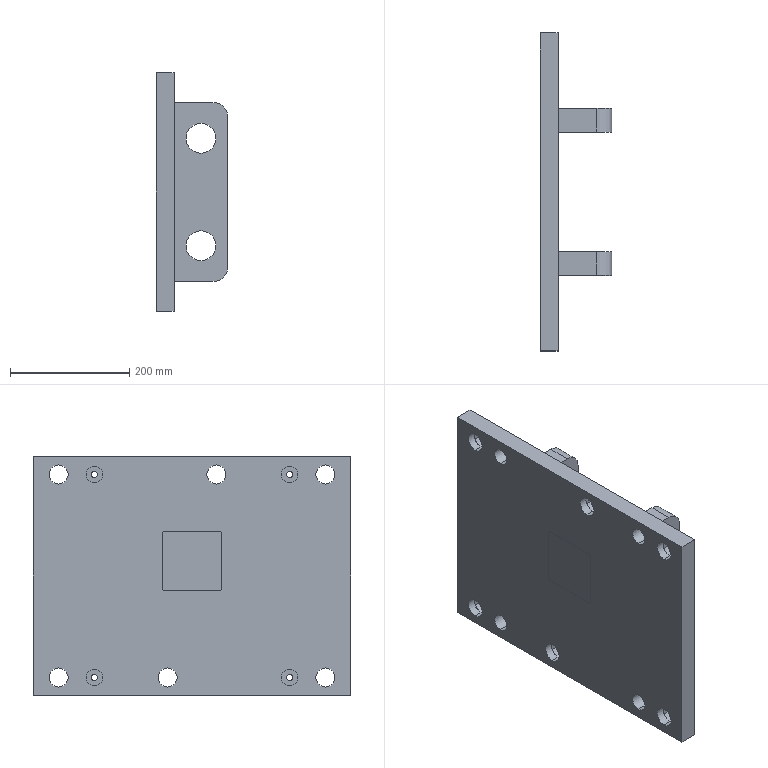Part | STEP file | LM-05-1233_default | 1 solid | 117 faces | box 120 x 532 x 400 mm | volume 7941008 mm3 | cylinder 62 | plane 43 | cone 12 | commonest cylinder face diameters 46 x18 10 x12 32 x12 50 x12 28 x8